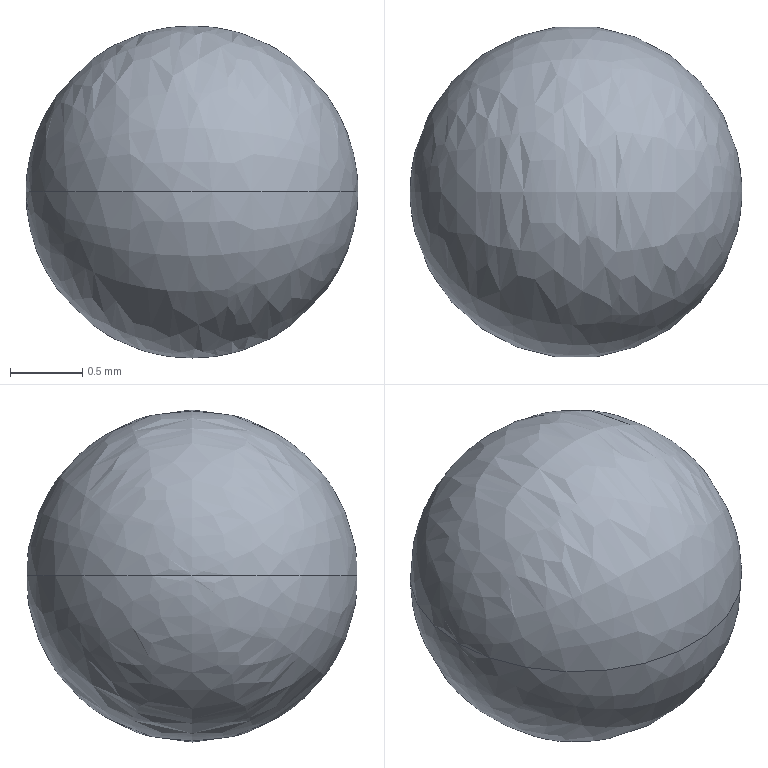Part | SolidWorks | features BaseBody 1 | 1 solid | 2 faces | volume 6.37 mm3 | spline 2